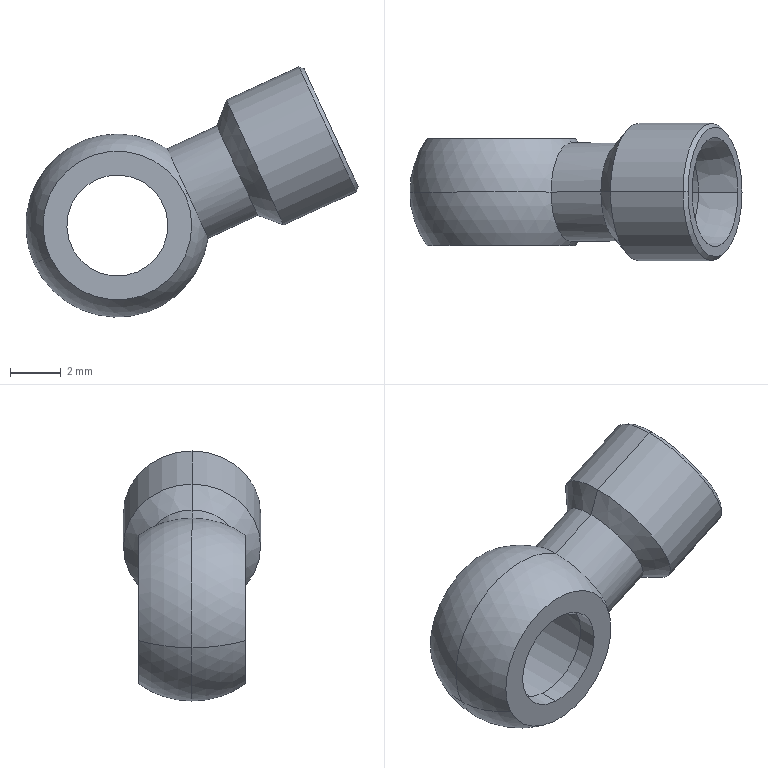Part | STEP file | 2026.6.15-Main Assembly图.sldasm-Part-257 | 1 solid | 31 faces | box 13.063 x 5.4 x 9.839 mm | volume 145.21 mm3 | cylinder 14 | cone 8 | plane 5 | sphere 4 | commonest cylinder face diameters 3.975 x4 2.1 x2 3.66 x2 3.87 x2 4.875 x2 5.4 x2
STEP:
#1=CARTESIAN_POINT('',(-1613.628,1444.049,3409.35));
#2=VERTEX_POINT('',#1);
#3=CARTESIAN_POINT('',(-1612.823,1442.114,3407.591));
#4=VERTEX_POINT('',#3);
#5=CARTESIAN_POINT('',(-1613.628,1442.114,3409.35));
#6=DIRECTION('',(-0.9092,0.,-0.4163));
#7=DIRECTION('',(0.4163,0.,-0.9092));
#8=AXIS2_PLACEMENT_3D('',#5,#6,#7);
#9=CIRCLE('',#8,1.935);
#10=EDGE_CURVE('',#2,#4,#9,.T.);
#11=ORIENTED_EDGE('',*,*,#10,.T.);
#12=CARTESIAN_POINT('',(-1619.662,1442.114,3406.588));
#13=VERTEX_POINT('',#12);
#14=CARTESIAN_POINT('',(-1616.388,1442.114,3408.086));
#15=DIRECTION('',(0.,1.,0.));
#16=DIRECTION('',(1.,0.,0.));
#17=AXIS2_PLACEMENT_3D('',#14,#15,#16);
#18=CIRCLE('',#17,3.6);
#19=EDGE_CURVE('',#4,#13,#18,.T.);
#20=ORIENTED_EDGE('',*,*,#19,.T.);
#21=CARTESIAN_POINT('',(-1619.047,1444.214,3406.869));
#22=VERTEX_POINT('',#21);
#23=CARTESIAN_POINT('',(-1616.388,1442.114,3408.086));
#24=DIRECTION('',(0.4163,0.,-0.9092));
#25=DIRECTION('',(0.9092,0.,0.4163));
#26=AXIS2_PLACEMENT_3D('',#23,#24,#25);
#27=CIRCLE('',#26,3.6);
#28=EDGE_CURVE('',#13,#22,#27,.T.);
#29=ORIENTED_EDGE('',*,*,#28,.T.);
#30=CARTESIAN_POINT('',(-1613.73,1444.214,3409.304));
#31=VERTEX_POINT('',#30);
#32=CARTESIAN_POINT('',(-1616.388,1444.214,3408.086));
#33=DIRECTION('',(0.,-1.,0.));
#34=DIRECTION('',(0.0785,0.,0.9969));
#35=AXIS2_PLACEMENT_3D('',#32,#33,#34);
#36=CIRCLE('',#35,2.924);
#37=EDGE_CURVE('',#22,#31,#36,.T.);
#38=ORIENTED_EDGE('',*,*,#37,.T.);
#39=CARTESIAN_POINT('',(-1616.388,1442.114,3408.086));
#40=DIRECTION('',(-0.4163,0.,0.9092));
#41=DIRECTION('',(-0.9092,0.,-0.4163));
#42=AXIS2_PLACEMENT_3D('',#39,#40,#41);
#43=CIRCLE('',#42,3.6);
#44=EDGE_CURVE('',#2,#31,#43,.T.);
#45=ORIENTED_EDGE('',*,*,#44,.F.);
#46=EDGE_LOOP('',(#11,#20,#29,#38,#45));
#47=FACE_OUTER_BOUND('',#46,.T.);
#48=CARTESIAN_POINT('',(-1616.388,1442.114,3408.086));
#49=DIRECTION('',(0.,1.,0.));
#50=DIRECTION('',(0.9092,0.,0.4163));
#51=AXIS2_PLACEMENT_3D('',#48,#49,#50);
#52=SPHERICAL_SURFACE('',#51,3.6);
#53=ADVANCED_FACE('',(#47),#52,.T.);
#54=CARTESIAN_POINT('',(-1614.434,1442.114,3411.109));
#55=VERTEX_POINT('',#54);
#56=CARTESIAN_POINT('',(-1616.388,1442.114,3408.086));
#57=DIRECTION('',(0.,-1.,0.));
#58=DIRECTION('',(0.,0.,1.));
#59=AXIS2_PLACEMENT_3D('',#56,#57,#58);
#60=CIRCLE('',#59,3.6);
#61=EDGE_CURVE('',#55,#13,#60,.T.);
#62=ORIENTED_EDGE('',*,*,#61,.F.);
#63=CARTESIAN_POINT('',(-1613.628,1442.114,3409.35));
#64=DIRECTION('',(-0.9092,0.,-0.4163));
#65=DIRECTION('',(0.4163,0.,-0.9092));
#66=AXIS2_PLACEMENT_3D('',#63,#64,#65);
#67=CIRCLE('',#66,1.935);
#68=EDGE_CURVE('',#55,#2,#67,.T.);
#69=ORIENTED_EDGE('',*,*,#68,.T.);
#70=ORIENTED_EDGE('',*,*,#44,.T.);
#71=CARTESIAN_POINT('',(-1616.388,1444.214,3408.086));
#72=DIRECTION('',(0.,-1.,0.));
#73=DIRECTION('',(0.0785,0.,0.9969));
#74=AXIS2_PLACEMENT_3D('',#71,#72,#73);
#75=CIRCLE('',#74,2.924);
#76=EDGE_CURVE('',#31,#22,#75,.T.);
#77=ORIENTED_EDGE('',*,*,#76,.T.);
#78=ORIENTED_EDGE('',*,*,#28,.F.);
#79=EDGE_LOOP('',(#62,#69,#70,#77,#78));
#80=FACE_OUTER_BOUND('',#79,.T.);
#81=CARTESIAN_POINT('',(-1616.388,1442.114,3408.086));
#82=DIRECTION('',(0.,1.,0.));
#83=DIRECTION('',(0.9092,0.,0.4163));
#84=AXIS2_PLACEMENT_3D('',#81,#82,#83);
#85=SPHERICAL_SURFACE('',#84,3.6);
#86=ADVANCED_FACE('',(#80),#85,.T.);
#87=CARTESIAN_POINT('',(-1611.067,1442.114,3412.535));
#88=VERTEX_POINT('',#87);
#89=CARTESIAN_POINT('',(-1610.16,1442.114,3412.95));
#90=VERTEX_POINT('',#89);
#91=CARTESIAN_POINT('',(-1610.16,1442.114,3412.95));
#92=DIRECTION('',(0.9092,0.,0.4163));
#93=VECTOR('',#92,1000.);
#94=LINE('',#91,#93);
#95=EDGE_CURVE('',#88,#90,#94,.T.);
#96=ORIENTED_EDGE('',*,*,#95,.F.);
#97=CARTESIAN_POINT('',(-1609.544,1442.114,3409.207));
#98=VERTEX_POINT('',#97);
#99=CARTESIAN_POINT('',(-1610.305,1442.114,3410.871));
#100=DIRECTION('',(-0.9092,0.,-0.4163));
#101=DIRECTION('',(0.4163,0.,-0.9092));
#102=AXIS2_PLACEMENT_3D('',#99,#100,#101);
#103=CIRCLE('',#102,1.83);
#104=EDGE_CURVE('',#88,#98,#103,.T.);
#105=ORIENTED_EDGE('',*,*,#104,.T.);
#106=CARTESIAN_POINT('',(-1608.637,1442.114,3409.623));
#107=VERTEX_POINT('',#106);
#108=CARTESIAN_POINT('',(-1608.637,1442.114,3409.623));
#109=DIRECTION('',(0.9092,0.,0.4163));
#110=VECTOR('',#109,1000.);
#111=LINE('',#108,#110);
#112=EDGE_CURVE('',#98,#107,#111,.T.);
#113=ORIENTED_EDGE('',*,*,#112,.T.);
#114=CARTESIAN_POINT('',(-1609.399,1442.114,3411.286));
#115=DIRECTION('',(0.9092,0.,0.4163));
#116=DIRECTION('',(0.4163,0.,-0.9092));
#117=AXIS2_PLACEMENT_3D('',#114,#115,#116);
#118=CIRCLE('',#117,1.83);
#119=EDGE_CURVE('',#107,#90,#118,.T.);
#120=ORIENTED_EDGE('',*,*,#119,.T.);
#121=EDGE_LOOP('',(#96,#105,#113,#120));
#122=FACE_OUTER_BOUND('',#121,.T.);
#123=CARTESIAN_POINT('',(-1609.399,1442.114,3411.286));
#124=DIRECTION('',(0.9092,0.,0.4163));
#125=DIRECTION('',(-0.4163,0.,0.9092));
#126=AXIS2_PLACEMENT_3D('',#123,#124,#125);
#127=CYLINDRICAL_SURFACE('',#126,1.83);
#128=ADVANCED_FACE('',(#122),#127,.F.);
#129=CARTESIAN_POINT('',(-1611.452,1442.114,3411.501));
#130=VERTEX_POINT('',#129);
#131=CARTESIAN_POINT('',(-1611.067,1442.114,3412.535));
#132=DIRECTION('',(0.3486,0.,0.9373));
#133=VECTOR('',#132,1000.);
#134=LINE('',#131,#133);
#135=EDGE_CURVE('',#130,#88,#134,.T.);
#136=ORIENTED_EDGE('',*,*,#135,.F.);
#137=CARTESIAN_POINT('',(-1610.578,1442.114,3409.592));
#138=VERTEX_POINT('',#137);
#139=CARTESIAN_POINT('',(-1611.015,1442.114,3410.547));
#140=DIRECTION('',(-0.9092,0.,-0.4163));
#141=DIRECTION('',(-0.4163,0.,0.9092));
#142=AXIS2_PLACEMENT_3D('',#139,#140,#141);
#143=CIRCLE('',#142,1.05);
#144=EDGE_CURVE('',#130,#138,#143,.T.);
#145=ORIENTED_EDGE('',*,*,#144,.T.);
#146=CARTESIAN_POINT('',(-1609.544,1442.114,3409.207));
#147=DIRECTION('',(0.9373,0.,-0.3486));
#148=VECTOR('',#147,1000.);
#149=LINE('',#146,#148);
#150=EDGE_CURVE('',#138,#98,#149,.T.);
#151=ORIENTED_EDGE('',*,*,#150,.T.);
#152=ORIENTED_EDGE('',*,*,#104,.F.);
#153=EDGE_LOOP('',(#136,#145,#151,#152));
#154=FACE_OUTER_BOUND('',#153,.T.);
#155=CARTESIAN_POINT('',(-1610.305,1442.114,3410.871));
#156=DIRECTION('',(0.9092,0.,0.4163));
#157=DIRECTION('',(-0.4163,0.,0.9092));
#158=AXIS2_PLACEMENT_3D('',#155,#156,#157);
#159=CONICAL_SURFACE('',#158,1.83,0.7854);
#160=ADVANCED_FACE('',(#154),#159,.F.);
#161=CARTESIAN_POINT('',(-1608.886,1442.114,3413.897));
#162=VERTEX_POINT('',#161);
#163=CARTESIAN_POINT('',(-1608.886,1442.114,3413.897));
#164=DIRECTION('',(0.8028,0.,0.5962));
#165=VECTOR('',#164,1000.);
#166=LINE('',#163,#165);
#167=EDGE_CURVE('',#90,#162,#166,.T.);
#168=ORIENTED_EDGE('',*,*,#167,.F.);
#169=ORIENTED_EDGE('',*,*,#119,.F.);
#170=CARTESIAN_POINT('',(-1607.088,1442.114,3409.969));
#171=VERTEX_POINT('',#170);
#172=CARTESIAN_POINT('',(-1607.088,1442.114,3409.969));
#173=DIRECTION('',(0.9759,0.,0.2181));
#174=VECTOR('',#173,1000.);
#175=LINE('',#172,#174);
#176=EDGE_CURVE('',#107,#171,#175,.T.);
#177=ORIENTED_EDGE('',*,*,#176,.T.);
#178=CARTESIAN_POINT('',(-1607.987,1442.114,3411.933));
#179=DIRECTION('',(-0.9092,0.,-0.4163));
#180=DIRECTION('',(0.4163,0.,-0.9092));
#181=AXIS2_PLACEMENT_3D('',#178,#179,#180);
#182=CIRCLE('',#181,2.16);
#183=EDGE_CURVE('',#162,#171,#182,.T.);
#184=ORIENTED_EDGE('',*,*,#183,.F.);
#185=EDGE_LOOP('',(#168,#169,#177,#184));
#186=FACE_OUTER_BOUND('',#185,.T.);
#187=CARTESIAN_POINT('',(-1607.987,1442.114,3411.933));
#188=DIRECTION('',(0.9092,0.,0.4163));
#189=DIRECTION('',(-0.4163,0.,0.9092));
#190=AXIS2_PLACEMENT_3D('',#187,#188,#189);
#191=CONICAL_SURFACE('',#190,2.16,0.2094);
#192=ADVANCED_FACE('',(#186),#191,.F.);
#193=CARTESIAN_POINT('',(-1613.951,1442.114,3408.047));
#194=VERTEX_POINT('',#193);
#195=CARTESIAN_POINT('',(-1621.807,1442.114,3404.451));
#196=DIRECTION('',(0.9092,0.,0.4163));
#197=VECTOR('',#196,1000.);
#198=LINE('',#195,#197);
#199=EDGE_CURVE('',#194,#138,#198,.T.);
#200=ORIENTED_EDGE('',*,*,#199,.T.);
#201=ORIENTED_EDGE('',*,*,#144,.F.);
#202=CARTESIAN_POINT('',(-1614.825,1442.114,3409.957));
#203=VERTEX_POINT('',#202);
#204=CARTESIAN_POINT('',(-1622.681,1442.114,3406.36));
#205=DIRECTION('',(0.9092,0.,0.4163));
#206=VECTOR('',#205,1000.);
#207=LINE('',#204,#206);
#208=EDGE_CURVE('',#203,#130,#207,.T.);
#209=ORIENTED_EDGE('',*,*,#208,.F.);
#210=CARTESIAN_POINT('',(-1614.825,1442.114,3409.957));
#211=CARTESIAN_POINT('',(-1614.825,1442.255,3409.957));
#212=CARTESIAN_POINT('',(-1614.801,1442.393,3409.937));
#213=CARTESIAN_POINT('',(-1614.715,1442.646,3409.86));
#214=CARTESIAN_POINT('',(-1614.654,1442.761,3409.802));
#215=CARTESIAN_POINT('',(-1614.519,1442.952,3409.654));
#216=CARTESIAN_POINT('',(-1614.444,1443.03,3409.561));
#217=CARTESIAN_POINT('',(-1614.3,1443.136,3409.35));
#218=CARTESIAN_POINT('',(-1614.231,1443.164,3409.229));
#219=CARTESIAN_POINT('',(-1614.115,1443.164,3408.976));
#220=CARTESIAN_POINT('',(-1614.068,1443.137,3408.845));
#221=CARTESIAN_POINT('',(-1614.001,1443.03,3408.594));
#222=CARTESIAN_POINT('',(-1613.98,1442.953,3408.478));
#223=CARTESIAN_POINT('',(-1613.956,1442.761,3408.278));
#224=CARTESIAN_POINT('',(-1613.952,1442.646,3408.194));
#225=CARTESIAN_POINT('',(-1613.95,1442.394,3408.079));
#226=CARTESIAN_POINT('',(-1613.951,1442.255,3408.047));
#227=CARTESIAN_POINT('',(-1613.951,1442.114,3408.047));
#228=B_SPLINE_CURVE_WITH_KNOTS('',3,(#210,#211,#212,#213,#214,#215,#216,#217,#218,#219,#220,#221,#222,#223,#224,#225,#226,#227),.UNSPECIFIED.,.F.,.F.,(4,2,2,2,2,2,2,2,4),(0.,0.0004153,0.0008305,0.001246,0.001661,0.002076,0.002492,0.002907,0.003322),.UNSPECIFIED.);
#229=EDGE_CURVE('',#203,#194,#228,.T.);
#230=ORIENTED_EDGE('',*,*,#229,.T.);
#231=EDGE_LOOP('',(#200,#201,#209,#230));
#232=FACE_OUTER_BOUND('',#231,.T.);
#233=CARTESIAN_POINT('',(-1622.244,1442.114,3405.405));
#234=DIRECTION('',(-0.9092,0.,-0.4163));
#235=DIRECTION('',(0.4163,0.,-0.9092));
#236=AXIS2_PLACEMENT_3D('',#233,#234,#235);
#237=CYLINDRICAL_SURFACE('',#236,1.05);
#238=ADVANCED_FACE('',(#232),#237,.F.);
#239=CARTESIAN_POINT('',(-1609.048,1442.114,3414.251));
#240=VERTEX_POINT('',#239);
#241=CARTESIAN_POINT('',(-1606.925,1442.114,3409.614));
#242=VERTEX_POINT('',#241);
#243=CARTESIAN_POINT('',(-1607.987,1442.114,3411.933));
#244=DIRECTION('',(-0.9092,0.,-0.4163));
#245=DIRECTION('',(-0.4163,0.,0.9092));
#246=AXIS2_PLACEMENT_3D('',#243,#244,#245);
#247=CIRCLE('',#246,2.55);
#248=EDGE_CURVE('',#240,#242,#247,.T.);
#249=ORIENTED_EDGE('',*,*,#248,.F.);
#250=CARTESIAN_POINT('',(-1607.987,1442.114,3411.933));
#251=DIRECTION('',(-0.9092,0.,-0.4163));
#252=DIRECTION('',(-0.4163,0.,0.9092));
#253=AXIS2_PLACEMENT_3D('',#250,#251,#252);
#254=CIRCLE('',#253,2.55);
#255=EDGE_CURVE('',#242,#240,#254,.T.);
#256=ORIENTED_EDGE('',*,*,#255,.F.);
#257=EDGE_LOOP('',(#249,#256));
#258=FACE_OUTER_BOUND('',#257,.T.);
#259=CARTESIAN_POINT('',(-1607.987,1442.114,3411.933));
#260=DIRECTION('',(-0.9092,0.,-0.4163));
#261=DIRECTION('',(0.4163,0.,-0.9092));
#262=AXIS2_PLACEMENT_3D('',#259,#260,#261);
#263=CIRCLE('',#262,2.16);
#264=EDGE_CURVE('',#171,#162,#263,.T.);
#265=ORIENTED_EDGE('',*,*,#264,.T.);
#266=ORIENTED_EDGE('',*,*,#183,.T.);
#267=EDGE_LOOP('',(#265,#266));
#268=FACE_BOUND('',#267,.T.);
#269=CARTESIAN_POINT('',(-1607.987,1444.814,3411.933));
#270=DIRECTION('',(0.9092,0.,0.4163));
#271=DIRECTION('',(-0.4163,0.,0.9092));
#272=AXIS2_PLACEMENT_3D('',#269,#270,#271);
#273=PLANE('',#272);
#274=ADVANCED_FACE('',(#258,#268),#273,.T.);
#275=CARTESIAN_POINT('',(-1616.197,1440.764,3410.516));
#276=VERTEX_POINT('',#275);
#277=CARTESIAN_POINT('',(-1616.197,1443.464,3410.516));
#278=VERTEX_POINT('',#277);
#279=CARTESIAN_POINT('',(-1616.197,1425.014,3410.516));
#280=DIRECTION('',(0.,1.,0.));
#281=VECTOR('',#280,1000.);
#282=LINE('',#279,#281);
#283=EDGE_CURVE('',#276,#278,#282,.T.);
#284=ORIENTED_EDGE('',*,*,#283,.F.);
#285=CARTESIAN_POINT('',(-1616.58,1440.764,3405.656));
#286=VERTEX_POINT('',#285);
#287=CARTESIAN_POINT('',(-1616.388,1440.764,3408.086));
#288=DIRECTION('',(0.,1.,0.));
#289=DIRECTION('',(-0.0785,0.,-0.9969));
#290=AXIS2_PLACEMENT_3D('',#287,#288,#289);
#291=CIRCLE('',#290,2.438);
#292=EDGE_CURVE('',#286,#276,#291,.T.);
#293=ORIENTED_EDGE('',*,*,#292,.F.);
#294=CARTESIAN_POINT('',(-1616.58,1443.464,3405.656));
#295=VERTEX_POINT('',#294);
#296=CARTESIAN_POINT('',(-1616.58,1425.014,3405.656));
#297=DIRECTION('',(0.,1.,0.));
#298=VECTOR('',#297,1000.);
#299=LINE('',#296,#298);
#300=EDGE_CURVE('',#286,#295,#299,.T.);
#301=ORIENTED_EDGE('',*,*,#300,.T.);
#302=CARTESIAN_POINT('',(-1616.388,1443.464,3408.086));
#303=DIRECTION('',(0.,-1.,0.));
#304=DIRECTION('',(-0.0785,0.,-0.9969));
#305=AXIS2_PLACEMENT_3D('',#302,#303,#304);
#306=CIRCLE('',#305,2.438);
#307=EDGE_CURVE('',#278,#295,#306,.T.);
#308=ORIENTED_EDGE('',*,*,#307,.F.);
#309=EDGE_LOOP('',(#284,#293,#301,#308));
#310=FACE_OUTER_BOUND('',#309,.T.);
#311=CARTESIAN_POINT('',(-1616.388,1425.014,3408.086));
#312=DIRECTION('',(0.,1.,0.));
#313=DIRECTION('',(0.0785,0.,0.9969));
#314=AXIS2_PLACEMENT_3D('',#311,#312,#313);
#315=CYLINDRICAL_SURFACE('',#314,2.438);
#316=ADVANCED_FACE('',(#310),#315,.F.);
#317=CARTESIAN_POINT('',(-1606.999,1442.114,3409.415));
#318=VERTEX_POINT('',#317);
#319=CARTESIAN_POINT('',(-1606.999,1442.114,3409.415));
#320=DIRECTION('',(0.3486,0.,0.9373));
#321=VECTOR('',#320,1000.);
#322=LINE('',#319,#321);
#323=EDGE_CURVE('',#318,#242,#322,.T.);
#324=ORIENTED_EDGE('',*,*,#323,.T.);
#325=ORIENTED_EDGE('',*,*,#255,.T.);
#326=CARTESIAN_POINT('',(-1609.247,1442.114,3414.325));
#327=VERTEX_POINT('',#326);
#328=CARTESIAN_POINT('',(-1609.247,1442.114,3414.325));
#329=DIRECTION('',(0.9373,0.,-0.3486));
#330=VECTOR('',#329,1000.);
#331=LINE('',#328,#330);
#332=EDGE_CURVE('',#327,#240,#331,.T.);
#333=ORIENTED_EDGE('',*,*,#332,.F.);
#334=CARTESIAN_POINT('',(-1608.123,1442.114,3411.87));
#335=DIRECTION('',(-0.9092,0.,-0.4163));
#336=DIRECTION('',(0.4163,0.,-0.9092));
#337=AXIS2_PLACEMENT_3D('',#334,#335,#336);
#338=CIRCLE('',#337,2.7);
#339=EDGE_CURVE('',#318,#327,#338,.T.);
#340=ORIENTED_EDGE('',*,*,#339,.F.);
#341=EDGE_LOOP('',(#324,#325,#333,#340));
#342=FACE_OUTER_BOUND('',#341,.T.);
#343=CARTESIAN_POINT('',(-1608.123,1442.114,3411.87));
#344=DIRECTION('',(-0.9092,0.,-0.4163));
#345=DIRECTION('',(0.4163,0.,-0.9092));
#346=AXIS2_PLACEMENT_3D('',#343,#344,#345);
#347=CONICAL_SURFACE('',#346,2.7,0.7854);
#348=ADVANCED_FACE('',(#342),#347,.T.);
#349=ORIENTED_EDGE('',*,*,#292,.T.);
#350=CARTESIAN_POINT('',(-1616.388,1440.764,3408.086));
#351=DIRECTION('',(0.,1.,0.));
#352=DIRECTION('',(-0.0785,0.,-0.9969));
#353=AXIS2_PLACEMENT_3D('',#350,#351,#352);
#354=CIRCLE('',#353,2.438);
#355=EDGE_CURVE('',#276,#286,#354,.T.);
#356=ORIENTED_EDGE('',*,*,#355,.T.);
#357=EDGE_LOOP('',(#349,#356));
#358=FACE_OUTER_BOUND('',#357,.T.);
#359=CARTESIAN_POINT('',(-1616.544,1440.764,3406.105));
#360=VERTEX_POINT('',#359);
#361=CARTESIAN_POINT('',(-1616.232,1440.764,3410.068));
#362=VERTEX_POINT('',#361);
#363=CARTESIAN_POINT('',(-1616.388,1440.764,3408.086));
#364=DIRECTION('',(0.,-1.,0.));
#365=DIRECTION('',(-0.0785,0.,-0.9969));
#366=AXIS2_PLACEMENT_3D('',#363,#364,#365);
#367=CIRCLE('',#366,1.987);
#368=EDGE_CURVE('',#360,#362,#367,.T.);
#369=ORIENTED_EDGE('',*,*,#368,.T.);
#370=CARTESIAN_POINT('',(-1616.388,1440.764,3408.086));
#371=DIRECTION('',(0.,-1.,0.));
#372=DIRECTION('',(-0.0785,0.,-0.9969));
#373=AXIS2_PLACEMENT_3D('',#370,#371,#372);
#374=CIRCLE('',#373,1.987);
#375=EDGE_CURVE('',#362,#360,#374,.T.);
#376=ORIENTED_EDGE('',*,*,#375,.T.);
#377=EDGE_LOOP('',(#369,#376));
#378=FACE_BOUND('',#377,.T.);
#379=CARTESIAN_POINT('',(-1617.403,1440.764,3410.303));
#380=DIRECTION('',(0.,1.,0.));
#381=DIRECTION('',(1.,0.,0.));
#382=AXIS2_PLACEMENT_3D('',#379,#380,#381);
#383=PLANE('',#382);
#384=ADVANCED_FACE('',(#358,#378),#383,.T.);
#385=CARTESIAN_POINT('',(-1616.388,1443.464,3408.086));
#386=DIRECTION('',(0.,-1.,0.));
#387=DIRECTION('',(-0.0785,0.,-0.9969));
#388=AXIS2_PLACEMENT_3D('',#385,#386,#387);
#389=CIRCLE('',#388,2.438);
#390=EDGE_CURVE('',#295,#278,#389,.T.);
#391=ORIENTED_EDGE('',*,*,#390,.T.);
#392=ORIENTED_EDGE('',*,*,#307,.T.);
#393=EDGE_LOOP('',(#391,#392));
#394=FACE_OUTER_BOUND('',#393,.T.);
#395=CARTESIAN_POINT('',(-1616.544,1443.464,3406.105));
#396=VERTEX_POINT('',#395);
#397=CARTESIAN_POINT('',(-1616.232,1443.464,3410.068));
#398=VERTEX_POINT('',#397);
#399=CARTESIAN_POINT('',(-1616.388,1443.464,3408.086));
#400=DIRECTION('',(0.,1.,0.));
#401=DIRECTION('',(-0.0785,0.,-0.9969));
#402=AXIS2_PLACEMENT_3D('',#399,#400,#401);
#403=CIRCLE('',#402,1.987);
#404=EDGE_CURVE('',#396,#398,#403,.T.);
#405=ORIENTED_EDGE('',*,*,#404,.T.);
#406=CARTESIAN_POINT('',(-1616.388,1443.464,3408.086));
#407=DIRECTION('',(0.,1.,0.));
#408=DIRECTION('',(-0.0785,0.,-0.9969));
#409=AXIS2_PLACEMENT_3D('',#406,#407,#408);
#410=CIRCLE('',#409,1.987);
#411=EDGE_CURVE('',#398,#396,#410,.T.);
#412=ORIENTED_EDGE('',*,*,#411,.T.);
#413=EDGE_LOOP('',(#405,#412));
#414=FACE_BOUND('',#413,.T.);
#415=CARTESIAN_POINT('',(-1617.216,1443.464,3409.893));
#416=DIRECTION('',(0.,-1.,0.));
#417=DIRECTION('',(0.,0.,-1.));
#418=AXIS2_PLACEMENT_3D('',#415,#416,#417);
#419=PLANE('',#418);
#420=ADVANCED_FACE('',(#394,#414),#419,.T.);
#421=CARTESIAN_POINT('',(-1612.098,1442.114,3413.02));
#422=VERTEX_POINT('',#421);
#423=CARTESIAN_POINT('',(-1633.878,1442.114,3403.048));
#424=DIRECTION('',(0.9092,0.,0.4163));
#425=VECTOR('',#424,1000.);
#426=LINE('',#423,#425);
#427=EDGE_CURVE('',#422,#327,#426,.T.);
#428=ORIENTED_EDGE('',*,*,#427,.F.);
#429=CARTESIAN_POINT('',(-1609.85,1442.114,3408.11));
#430=VERTEX_POINT('',#429);
#431=CARTESIAN_POINT('',(-1610.974,1442.114,3410.565));
#432=DIRECTION('',(-0.9092,0.,-0.4163));
#433=DIRECTION('',(0.4163,0.,-0.9092));
#434=AXIS2_PLACEMENT_3D('',#431,#432,#433);
#435=CIRCLE('',#434,2.7);
#436=EDGE_CURVE('',#430,#422,#435,.T.);
#437=ORIENTED_EDGE('',*,*,#436,.F.);
#438=CARTESIAN_POINT('',(-1631.631,1442.114,3398.138));
#439=DIRECTION('',(0.9092,0.,0.4163));
#440=VECTOR('',#439,1000.);
#441=LINE('',#438,#440);
#442=EDGE_CURVE('',#430,#318,#441,.T.);
#443=ORIENTED_EDGE('',*,*,#442,.T.);
#444=ORIENTED_EDGE('',*,*,#339,.T.);
#445=EDGE_LOOP('',(#428,#437,#443,#444));
#446=FACE_OUTER_BOUND('',#445,.T.);
#447=CARTESIAN_POINT('',(-1632.755,1442.114,3400.593));
#448=DIRECTION('',(0.9092,0.,0.4163));
#449=DIRECTION('',(-0.4163,0.,0.9092));
#450=AXIS2_PLACEMENT_3D('',#447,#448,#449);
#451=CYLINDRICAL_SURFACE('',#450,2.7);
#452=ADVANCED_FACE('',(#446),#451,.T.);
#453=CARTESIAN_POINT('',(-1616.232,1440.014,3410.068));
#454=VERTEX_POINT('',#453);
#455=CARTESIAN_POINT('',(-1616.232,1425.014,3410.068));
#456=DIRECTION('',(0.,1.,0.));
#457=VECTOR('',#456,1000.);
#458=LINE('',#455,#457);
#459=EDGE_CURVE('',#454,#362,#458,.T.);
#460=ORIENTED_EDGE('',*,*,#459,.F.);
#461=CARTESIAN_POINT('',(-1616.544,1440.014,3406.105));
#462=VERTEX_POINT('',#461);
#463=CARTESIAN_POINT('',(-1616.388,1440.014,3408.086));
#464=DIRECTION('',(0.,1.,0.));
#465=DIRECTION('',(-0.0785,0.,-0.9969));
#466=AXIS2_PLACEMENT_3D('',#463,#464,#465);
#467=CIRCLE('',#466,1.987);
#468=EDGE_CURVE('',#462,#454,#467,.T.);
#469=ORIENTED_EDGE('',*,*,#468,.F.);
#470=CARTESIAN_POINT('',(-1616.544,1425.014,3406.105));
#471=DIRECTION('',(0.,1.,0.));
#472=VECTOR('',#471,1000.);
#473=LINE('',#470,#472);
#474=EDGE_CURVE('',#462,#360,#473,.T.);
#475=ORIENTED_EDGE('',*,*,#474,.T.);
#476=ORIENTED_EDGE('',*,*,#375,.F.);
#477=EDGE_LOOP('',(#460,#469,#475,#476));
#478=FACE_OUTER_BOUND('',#477,.T.);
#479=CARTESIAN_POINT('',(-1616.388,1425.014,3408.086));
#480=DIRECTION('',(0.,1.,0.));
#481=DIRECTION('',(0.0785,0.,0.9969));
#482=AXIS2_PLACEMENT_3D('',#479,#480,#481);
#483=CYLINDRICAL_SURFACE('',#482,1.987);
#484=ADVANCED_FACE('',(#478),#483,.F.);
#485=CARTESIAN_POINT('',(-1616.232,1444.214,3410.068));
#486=VERTEX_POINT('',#485);
#487=CARTESIAN_POINT('',(-1616.232,1425.014,3410.068));
#488=DIRECTION('',(0.,1.,0.));
#489=VECTOR('',#488,1000.);
#490=LINE('',#487,#489);
#491=EDGE_CURVE('',#398,#486,#490,.T.);
#492=ORIENTED_EDGE('',*,*,#491,.F.);
#493=ORIENTED_EDGE('',*,*,#404,.F.);
#494=CARTESIAN_POINT('',(-1616.544,1444.214,3406.105));
#495=VERTEX_POINT('',#494);
#496=CARTESIAN_POINT('',(-1616.544,1425.014,3406.105));
#497=DIRECTION('',(0.,1.,0.));
#498=VECTOR('',#497,1000.);
#499=LINE('',#496,#498);
#500=EDGE_CURVE('',#396,#495,#499,.T.);
#501=ORIENTED_EDGE('',*,*,#500,.T.);
#502=CARTESIAN_POINT('',(-1616.388,1444.214,3408.086));
#503=DIRECTION('',(0.,-1.,0.));
#504=DIRECTION('',(-0.0785,0.,-0.9969));
#505=AXIS2_PLACEMENT_3D('',#502,#503,#504);
#506=CIRCLE('',#505,1.987);
#507=EDGE_CURVE('',#486,#495,#506,.T.);
#508=ORIENTED_EDGE('',*,*,#507,.F.);
#509=EDGE_LOOP('',(#492,#493,#501,#508));
#510=FACE_OUTER_BOUND('',#509,.T.);
#511=CARTESIAN_POINT('',(-1616.388,1425.014,3408.086));
#512=DIRECTION('',(0.,1.,0.));
#513=DIRECTION('',(0.0785,0.,0.9969));
#514=AXIS2_PLACEMENT_3D('',#511,#512,#513);
#515=CYLINDRICAL_SURFACE('',#514,1.987);
#516=ADVANCED_FACE('',(#510),#515,.F.);
#517=CARTESIAN_POINT('',(-1612.475,1442.114,3412.006));
#518=VERTEX_POINT('',#517);
#519=CARTESIAN_POINT('',(-1612.098,1442.114,3413.02));
#520=DIRECTION('',(0.3486,0.,0.9373));
#521=VECTOR('',#520,1000.);
#522=LINE('',#519,#521);
#523=EDGE_CURVE('',#518,#422,#522,.T.);
#524=ORIENTED_EDGE('',*,*,#523,.F.);
#525=CARTESIAN_POINT('',(-1610.864,1442.114,3408.487));
#526=VERTEX_POINT('',#525);
#527=CARTESIAN_POINT('',(-1611.669,1442.114,3410.247));
#528=DIRECTION('',(-0.9092,0.,-0.4163));
#529=DIRECTION('',(0.4163,0.,-0.9092));
#530=AXIS2_PLACEMENT_3D('',#527,#528,#529);
#531=CIRCLE('',#530,1.935);
#532=EDGE_CURVE('',#526,#518,#531,.T.);
#533=ORIENTED_EDGE('',*,*,#532,.F.);
#534=CARTESIAN_POINT('',(-1609.85,1442.114,3408.11));
#535=DIRECTION('',(0.9373,0.,-0.3486));
#536=VECTOR('',#535,1000.);
#537=LINE('',#534,#536);
#538=EDGE_CURVE('',#526,#430,#537,.T.);
#539=ORIENTED_EDGE('',*,*,#538,.T.);
#540=ORIENTED_EDGE('',*,*,#436,.T.);
#541=EDGE_LOOP('',(#524,#533,#539,#540));
#542=FACE_OUTER_BOUND('',#541,.T.);
#543=CARTESIAN_POINT('',(-1610.974,1442.114,3410.565));
#544=DIRECTION('',(0.9092,0.,0.4163));
#545=DIRECTION('',(-0.4163,0.,0.9092));
#546=AXIS2_PLACEMENT_3D('',#543,#544,#545);
#547=CONICAL_SURFACE('',#546,2.7,0.7854);
#548=ADVANCED_FACE('',(#542),#547,.T.);
#549=CARTESIAN_POINT('',(-1619.047,1440.014,3406.869));
#550=VERTEX_POINT('',#549);
#551=CARTESIAN_POINT('',(-1613.73,1440.014,3409.304));
#552=VERTEX_POINT('',#551);
#553=CARTESIAN_POINT('',(-1616.388,1440.014,3408.086));
#554=DIRECTION('',(0.,1.,0.));
#555=DIRECTION('',(0.0785,0.,0.9969));
#556=AXIS2_PLACEMENT_3D('',#553,#554,#555);
#557=CIRCLE('',#556,2.924);
#558=EDGE_CURVE('',#550,#552,#557,.T.);
#559=ORIENTED_EDGE('',*,*,#558,.F.);
#560=CARTESIAN_POINT('',(-1616.388,1440.014,3408.086));
#561=DIRECTION('',(0.,1.,0.));
#562=DIRECTION('',(0.0785,0.,0.9969));
#563=AXIS2_PLACEMENT_3D('',#560,#561,#562);
#564=CIRCLE('',#563,2.924);
#565=EDGE_CURVE('',#552,#550,#564,.T.);
#566=ORIENTED_EDGE('',*,*,#565,.F.);
#567=EDGE_LOOP('',(#559,#566));
#568=FACE_OUTER_BOUND('',#567,.T.);
#569=ORIENTED_EDGE('',*,*,#468,.T.);
#570=CARTESIAN_POINT('',(-1616.388,1440.014,3408.086));
#571=DIRECTION('',(0.,1.,0.));
#572=DIRECTION('',(-0.0785,0.,-0.9969));
#573=AXIS2_PLACEMENT_3D('',#570,#571,#572);
#574=CIRCLE('',#573,1.987);
#575=EDGE_CURVE('',#454,#462,#574,.T.);
#576=ORIENTED_EDGE('',*,*,#575,.T.);
#577=EDGE_LOOP('',(#569,#576));
#578=FACE_BOUND('',#577,.T.);
#579=CARTESIAN_POINT('',(-1616.38,1440.014,3427.607));
#580=DIRECTION('',(0.,-1.,0.));
#581=DIRECTION('',(0.,0.,-1.));
#582=AXIS2_PLACEMENT_3D('',#579,#580,#581);
#583=PLANE('',#582);
#584=ADVANCED_FACE('',(#568,#578),#583,.T.);
#585=ORIENTED_EDGE('',*,*,#37,.F.);
#586=ORIENTED_EDGE('',*,*,#76,.F.);
#587=EDGE_LOOP('',(#585,#586));
#588=FACE_OUTER_BOUND('',#587,.T.);
#589=CARTESIAN_POINT('',(-1616.388,1444.214,3408.086));
#590=DIRECTION('',(0.,-1.,0.));
#591=DIRECTION('',(-0.0785,0.,-0.9969));
#592=AXIS2_PLACEMENT_3D('',#589,#590,#591);
#593=CIRCLE('',#592,1.987);
#594=EDGE_CURVE('',#495,#486,#593,.T.);
#595=ORIENTED_EDGE('',*,*,#594,.T.);
#596=ORIENTED_EDGE('',*,*,#507,.T.);
#597=EDGE_LOOP('',(#595,#596));
#598=FACE_BOUND('',#597,.T.);
#599=CARTESIAN_POINT('',(-1630.41,1444.214,3421.775));
#600=DIRECTION('',(0.,1.,0.));
#601=DIRECTION('',(1.,0.,0.));
#602=AXIS2_PLACEMENT_3D('',#599,#600,#601);
#603=PLANE('',#602);
#604=ADVANCED_FACE('',(#588,#598),#603,.T.);
#605=CARTESIAN_POINT('',(-1633.56,1442.114,3402.353));
#606=DIRECTION('',(0.9092,0.,0.4163));
#607=VECTOR('',#606,1000.);
#608=LINE('',#605,#607);
#609=EDGE_CURVE('',#55,#518,#608,.T.);
#610=ORIENTED_EDGE('',*,*,#609,.F.);
#611=CARTESIAN_POINT('',(-1613.628,1440.179,3409.35));
#612=VERTEX_POINT('',#611);
#613=CARTESIAN_POINT('',(-1613.628,1442.114,3409.35));
#614=DIRECTION('',(-0.9092,0.,-0.4163));
#615=DIRECTION('',(0.4163,0.,-0.9092));
#616=AXIS2_PLACEMENT_3D('',#613,#614,#615);
#617=CIRCLE('',#616,1.935);
#618=EDGE_CURVE('',#612,#55,#617,.T.);
#619=ORIENTED_EDGE('',*,*,#618,.F.);
#620=CARTESIAN_POINT('',(-1613.628,1442.114,3409.35));
#621=DIRECTION('',(-0.9092,0.,-0.4163));
#622=DIRECTION('',(0.4163,0.,-0.9092));
#623=AXIS2_PLACEMENT_3D('',#620,#621,#622);
#624=CIRCLE('',#623,1.935);
#625=EDGE_CURVE('',#4,#612,#624,.T.);
#626=ORIENTED_EDGE('',*,*,#625,.F.);
#627=CARTESIAN_POINT('',(-1631.949,1442.114,3398.834));
#628=DIRECTION('',(0.9092,0.,0.4163));
#629=VECTOR('',#628,1000.);
#630=LINE('',#627,#629);
#631=EDGE_CURVE('',#4,#526,#630,.T.);
#632=ORIENTED_EDGE('',*,*,#631,.T.);
#633=ORIENTED_EDGE('',*,*,#532,.T.);
#634=EDGE_LOOP('',(#610,#619,#626,#632,#633));
#635=FACE_OUTER_BOUND('',#634,.T.);
#636=CARTESIAN_POINT('',(-1632.755,1442.114,3400.593));
#637=DIRECTION('',(0.9092,0.,0.4163));
#638=DIRECTION('',(-0.4163,0.,0.9092));
#639=AXIS2_PLACEMENT_3D('',#636,#637,#638);
#640=CYLINDRICAL_SURFACE('',#639,1.935);
#641=ADVANCED_FACE('',(#635),#640,.T.);
#642=ORIENTED_EDGE('',*,*,#618,.T.);
#643=ORIENTED_EDGE('',*,*,#61,.T.);
#644=CARTESIAN_POINT('',(-1616.388,1442.114,3408.086));
#645=DIRECTION('',(-0.4163,0.,0.9092));
#646=DIRECTION('',(0.9092,0.,0.4163));
#647=AXIS2_PLACEMENT_3D('',#644,#645,#646);
#648=CIRCLE('',#647,3.6);
#649=EDGE_CURVE('',#13,#550,#648,.T.);
#650=ORIENTED_EDGE('',*,*,#649,.T.);
#651=ORIENTED_EDGE('',*,*,#558,.T.);
#652=CARTESIAN_POINT('',(-1616.388,1442.114,3408.086));
#653=DIRECTION('',(0.4163,0.,-0.9092));
#654=DIRECTION('',(-0.9092,0.,-0.4163));
#655=AXIS2_PLACEMENT_3D('',#652,#653,#654);
#656=CIRCLE('',#655,3.6);
#657=EDGE_CURVE('',#612,#552,#656,.T.);
#658=ORIENTED_EDGE('',*,*,#657,.F.);
#659=EDGE_LOOP('',(#642,#643,#650,#651,#658));
#660=FACE_OUTER_BOUND('',#659,.T.);
#661=CARTESIAN_POINT('',(-1616.388,1442.114,3408.086));
#662=DIRECTION('',(0.,1.,0.));
#663=DIRECTION('',(0.9092,0.,0.4163));
#664=AXIS2_PLACEMENT_3D('',#661,#662,#663);
#665=SPHERICAL_SURFACE('',#664,3.6);
#666=ADVANCED_FACE('',(#660),#665,.T.);
#667=CARTESIAN_POINT('',(-1610.305,1442.114,3410.871));
#668=DIRECTION('',(-0.9092,0.,-0.4163));
#669=DIRECTION('',(0.4163,0.,-0.9092));
#670=AXIS2_PLACEMENT_3D('',#667,#668,#669);
#671=CIRCLE('',#670,1.83);
#672=EDGE_CURVE('',#98,#88,#671,.T.);
#673=ORIENTED_EDGE('',*,*,#672,.T.);
#674=ORIENTED_EDGE('',*,*,#95,.T.);
#675=CARTESIAN_POINT('',(-1609.399,1442.114,3411.286));
#676=DIRECTION('',(0.9092,0.,0.4163));
#677=DIRECTION('',(0.4163,0.,-0.9092));
#678=AXIS2_PLACEMENT_3D('',#675,#676,#677);
#679=CIRCLE('',#678,1.83);
#680=EDGE_CURVE('',#90,#107,#679,.T.);
#681=ORIENTED_EDGE('',*,*,#680,.T.);
#682=ORIENTED_EDGE('',*,*,#112,.F.);
#683=EDGE_LOOP('',(#673,#674,#681,#682));
#684=FACE_OUTER_BOUND('',#683,.T.);
#685=CARTESIAN_POINT('',(-1609.399,1442.114,3411.286));
#686=DIRECTION('',(0.9092,0.,0.4163));
#687=DIRECTION('',(-0.4163,0.,0.9092));
#688=AXIS2_PLACEMENT_3D('',#685,#686,#687);
#689=CYLINDRICAL_SURFACE('',#688,1.83);
#690=ADVANCED_FACE('',(#684),#689,.F.);
#691=CARTESIAN_POINT('',(-1611.015,1442.114,3410.547));
#692=DIRECTION('',(-0.9092,0.,-0.4163));
#693=DIRECTION('',(-0.4163,0.,0.9092));
#694=AXIS2_PLACEMENT_3D('',#691,#692,#693);
#695=CIRCLE('',#694,1.05);
#696=EDGE_CURVE('',#138,#130,#695,.T.);
#697=ORIENTED_EDGE('',*,*,#696,.T.);
#698=ORIENTED_EDGE('',*,*,#135,.T.);
#699=ORIENTED_EDGE('',*,*,#672,.F.);
#700=ORIENTED_EDGE('',*,*,#150,.F.);
#701=EDGE_LOOP('',(#697,#698,#699,#700));
#702=FACE_OUTER_BOUND('',#701,.T.);
#703=CARTESIAN_POINT('',(-1610.305,1442.114,3410.871));
#704=DIRECTION('',(0.9092,0.,0.4163));
#705=DIRECTION('',(-0.4163,0.,0.9092));
#706=AXIS2_PLACEMENT_3D('',#703,#704,#705);
#707=CONICAL_SURFACE('',#706,1.83,0.7854);
#708=ADVANCED_FACE('',(#702),#707,.F.);
#709=ORIENTED_EDGE('',*,*,#680,.F.);
#710=ORIENTED_EDGE('',*,*,#167,.T.);
#711=ORIENTED_EDGE('',*,*,#264,.F.);
#712=ORIENTED_EDGE('',*,*,#176,.F.);
#713=EDGE_LOOP('',(#709,#710,#711,#712));
#714=FACE_OUTER_BOUND('',#713,.T.);
#715=CARTESIAN_POINT('',(-1607.987,1442.114,3411.933));
#716=DIRECTION('',(0.9092,0.,0.4163));
#717=DIRECTION('',(-0.4163,0.,0.9092));
#718=AXIS2_PLACEMENT_3D('',#715,#716,#717);
#719=CONICAL_SURFACE('',#718,2.16,0.2094);
#720=ADVANCED_FACE('',(#714),#719,.F.);
#721=ORIENTED_EDGE('',*,*,#696,.F.);
#722=ORIENTED_EDGE('',*,*,#199,.F.);
#723=CARTESIAN_POINT('',(-1613.951,1442.114,3408.047));
#724=CARTESIAN_POINT('',(-1613.951,1441.974,3408.047));
#725=CARTESIAN_POINT('',(-1613.95,1441.836,3408.079));
#726=CARTESIAN_POINT('',(-1613.952,1441.583,3408.194));
#727=CARTESIAN_POINT('',(-1613.956,1441.468,3408.278));
#728=CARTESIAN_POINT('',(-1613.98,1441.277,3408.477));
#729=CARTESIAN_POINT('',(-1614.001,1441.199,3408.595));
#730=CARTESIAN_POINT('',(-1614.067,1441.093,3408.842));
#731=CARTESIAN_POINT('',(-1614.114,1441.064,3408.973));
#732=CARTESIAN_POINT('',(-1614.229,1441.064,3409.226));
#733=CARTESIAN_POINT('',(-1614.298,1441.092,3409.347));
#734=CARTESIAN_POINT('',(-1614.444,1441.199,3409.562));
#735=CARTESIAN_POINT('',(-1614.519,1441.276,3409.654));
#736=CARTESIAN_POINT('',(-1614.654,1441.468,3409.802));
#737=CARTESIAN_POINT('',(-1614.715,1441.583,3409.86));
#738=CARTESIAN_POINT('',(-1614.8,1441.835,3409.937));
#739=CARTESIAN_POINT('',(-1614.825,1441.974,3409.957));
#740=CARTESIAN_POINT('',(-1614.825,1442.114,3409.957));
#741=B_SPLINE_CURVE_WITH_KNOTS('',3,(#723,#724,#725,#726,#727,#728,#729,#730,#731,#732,#733,#734,#735,#736,#737,#738,#739,#740),.UNSPECIFIED.,.F.,.F.,(4,2,2,2,2,2,2,2,4),(0.,0.0004153,0.0008305,0.001246,0.001661,0.002076,0.002492,0.002907,0.003322),.UNSPECIFIED.);
#742=EDGE_CURVE('',#194,#203,#741,.T.);
#743=ORIENTED_EDGE('',*,*,#742,.T.);
#744=ORIENTED_EDGE('',*,*,#208,.T.);
#745=EDGE_LOOP('',(#721,#722,#743,#744));
#746=FACE_OUTER_BOUND('',#745,.T.);
#747=CARTESIAN_POINT('',(-1622.244,1442.114,3405.405));
#748=DIRECTION('',(-0.9092,0.,-0.4163));
#749=DIRECTION('',(0.4163,0.,-0.9092));
#750=AXIS2_PLACEMENT_3D('',#747,#748,#749);
#751=CYLINDRICAL_SURFACE('',#750,1.05);
#752=ADVANCED_FACE('',(#746),#751,.F.);
#753=ORIENTED_EDGE('',*,*,#355,.F.);
#754=ORIENTED_EDGE('',*,*,#283,.T.);
#755=ORIENTED_EDGE('',*,*,#390,.F.);
#756=ORIENTED_EDGE('',*,*,#300,.F.);
#757=EDGE_LOOP('',(#753,#754,#755,#756));
#758=FACE_OUTER_BOUND('',#757,.T.);
#759=ORIENTED_EDGE('',*,*,#229,.F.);
#760=ORIENTED_EDGE('',*,*,#742,.F.);
#761=EDGE_LOOP('',(#759,#760));
#762=FACE_BOUND('',#761,.T.);
#763=CARTESIAN_POINT('',(-1616.388,1425.014,3408.086));
#764=DIRECTION('',(0.,1.,0.));
#765=DIRECTION('',(0.0785,0.,0.9969));
#766=AXIS2_PLACEMENT_3D('',#763,#764,#765);
#767=CYLINDRICAL_SURFACE('',#766,2.438);
#768=ADVANCED_FACE('',(#758,#762),#767,.F.);
#769=ORIENTED_EDGE('',*,*,#248,.T.);
#770=ORIENTED_EDGE('',*,*,#323,.F.);
#771=CARTESIAN_POINT('',(-1608.123,1442.114,3411.87));
#772=DIRECTION('',(-0.9092,0.,-0.4163));
#773=DIRECTION('',(0.4163,0.,-0.9092));
#774=AXIS2_PLACEMENT_3D('',#771,#772,#773);
#775=CIRCLE('',#774,2.7);
#776=EDGE_CURVE('',#327,#318,#775,.T.);
#777=ORIENTED_EDGE('',*,*,#776,.F.);
#778=ORIENTED_EDGE('',*,*,#332,.T.);
#779=EDGE_LOOP('',(#769,#770,#777,#778));
#780=FACE_OUTER_BOUND('',#779,.T.);
#781=CARTESIAN_POINT('',(-1608.123,1442.114,3411.87));
#782=DIRECTION('',(-0.9092,0.,-0.4163));
#783=DIRECTION('',(0.4163,0.,-0.9092));
#784=AXIS2_PLACEMENT_3D('',#781,#782,#783);
#785=CONICAL_SURFACE('',#784,2.7,0.7854);
#786=ADVANCED_FACE('',(#780),#785,.T.);
#787=CARTESIAN_POINT('',(-1610.974,1442.114,3410.565));
#788=DIRECTION('',(-0.9092,0.,-0.4163));
#789=DIRECTION('',(0.4163,0.,-0.9092));
#790=AXIS2_PLACEMENT_3D('',#787,#788,#789);
#791=CIRCLE('',#790,2.7);
#792=EDGE_CURVE('',#422,#430,#791,.T.);
#793=ORIENTED_EDGE('',*,*,#792,.F.);
#794=ORIENTED_EDGE('',*,*,#427,.T.);
#795=ORIENTED_EDGE('',*,*,#776,.T.);
#796=ORIENTED_EDGE('',*,*,#442,.F.);
#797=EDGE_LOOP('',(#793,#794,#795,#796));
#798=FACE_OUTER_BOUND('',#797,.T.);
#799=CARTESIAN_POINT('',(-1632.755,1442.114,3400.593));
#800=DIRECTION('',(0.9092,0.,0.4163));
#801=DIRECTION('',(-0.4163,0.,0.9092));
#802=AXIS2_PLACEMENT_3D('',#799,#800,#801);
#803=CYLINDRICAL_SURFACE('',#802,2.7);
#804=ADVANCED_FACE('',(#798),#803,.T.);
#805=ORIENTED_EDGE('',*,*,#575,.F.);
#806=ORIENTED_EDGE('',*,*,#459,.T.);
#807=ORIENTED_EDGE('',*,*,#368,.F.);
#808=ORIENTED_EDGE('',*,*,#474,.F.);
#809=EDGE_LOOP('',(#805,#806,#807,#808));
#810=FACE_OUTER_BOUND('',#809,.T.);
#811=CARTESIAN_POINT('',(-1616.388,1425.014,3408.086));
#812=DIRECTION('',(0.,1.,0.));
#813=DIRECTION('',(0.0785,0.,0.9969));
#814=AXIS2_PLACEMENT_3D('',#811,#812,#813);
#815=CYLINDRICAL_SURFACE('',#814,1.987);
#816=ADVANCED_FACE('',(#810),#815,.F.);
#817=ORIENTED_EDGE('',*,*,#411,.F.);
#818=ORIENTED_EDGE('',*,*,#491,.T.);
#819=ORIENTED_EDGE('',*,*,#594,.F.);
#820=ORIENTED_EDGE('',*,*,#500,.F.);
#821=EDGE_LOOP('',(#817,#818,#819,#820));
#822=FACE_OUTER_BOUND('',#821,.T.);
#823=CARTESIAN_POINT('',(-1616.388,1425.014,3408.086));
#824=DIRECTION('',(0.,1.,0.));
#825=DIRECTION('',(0.0785,0.,0.9969));
#826=AXIS2_PLACEMENT_3D('',#823,#824,#825);
#827=CYLINDRICAL_SURFACE('',#826,1.987);
#828=ADVANCED_FACE('',(#822),#827,.F.);
#829=CARTESIAN_POINT('',(-1611.669,1442.114,3410.247));
#830=DIRECTION('',(-0.9092,0.,-0.4163));
#831=DIRECTION('',(0.4163,0.,-0.9092));
#832=AXIS2_PLACEMENT_3D('',#829,#830,#831);
#833=CIRCLE('',#832,1.935);
#834=EDGE_CURVE('',#518,#526,#833,.T.);
#835=ORIENTED_EDGE('',*,*,#834,.F.);
#836=ORIENTED_EDGE('',*,*,#523,.T.);
#837=ORIENTED_EDGE('',*,*,#792,.T.);
#838=ORIENTED_EDGE('',*,*,#538,.F.);
#839=EDGE_LOOP('',(#835,#836,#837,#838));
#840=FACE_OUTER_BOUND('',#839,.T.);
#841=CARTESIAN_POINT('',(-1610.974,1442.114,3410.565));
#842=DIRECTION('',(0.9092,0.,0.4163));
#843=DIRECTION('',(-0.4163,0.,0.9092));
#844=AXIS2_PLACEMENT_3D('',#841,#842,#843);
#845=CONICAL_SURFACE('',#844,2.7,0.7854);
#846=ADVANCED_FACE('',(#840),#845,.T.);
#847=ORIENTED_EDGE('',*,*,#68,.F.);
#848=ORIENTED_EDGE('',*,*,#609,.T.);
#849=ORIENTED_EDGE('',*,*,#834,.T.);
#850=ORIENTED_EDGE('',*,*,#631,.F.);
#851=ORIENTED_EDGE('',*,*,#10,.F.);
#852=EDGE_LOOP('',(#847,#848,#849,#850,#851));
#853=FACE_OUTER_BOUND('',#852,.T.);
#854=CARTESIAN_POINT('',(-1632.755,1442.114,3400.593));
#855=DIRECTION('',(0.9092,0.,0.4163));
#856=DIRECTION('',(-0.4163,0.,0.9092));
#857=AXIS2_PLACEMENT_3D('',#854,#855,#856);
#858=CYLINDRICAL_SURFACE('',#857,1.935);
#859=ADVANCED_FACE('',(#853),#858,.T.);
#860=ORIENTED_EDGE('',*,*,#19,.F.);
#861=ORIENTED_EDGE('',*,*,#625,.T.);
#862=ORIENTED_EDGE('',*,*,#657,.T.);
#863=ORIENTED_EDGE('',*,*,#565,.T.);
#864=ORIENTED_EDGE('',*,*,#649,.F.);
#865=EDGE_LOOP('',(#860,#861,#862,#863,#864));
#866=FACE_OUTER_BOUND('',#865,.T.);
#867=CARTESIAN_POINT('',(-1616.388,1442.114,3408.086));
#868=DIRECTION('',(0.,1.,0.));
#869=DIRECTION('',(0.9092,0.,0.4163));
#870=AXIS2_PLACEMENT_3D('',#867,#868,#869);
#871=SPHERICAL_SURFACE('',#870,3.6);
#872=ADVANCED_FACE('',(#866),#871,.T.);
#873=CLOSED_SHELL('',(#53,#86,#128,#160,#192,#238,#274,#316,#348,#384,#420,#452,#484,#516,#548,#584,#604,#641,#666,#690,#708,#720,#752,#768,#786,#804,#816,#828,#846,#859,#872));
#874=MANIFOLD_SOLID_BREP('',#873);
#875=CARTESIAN_POINT('',(0.,0.,0.));
#876=DIRECTION('',(0.,0.,1.));
#877=DIRECTION('',(1.,0.,0.));
#878=AXIS2_PLACEMENT_3D('',#875,#876,#877);
#879=(LENGTH_UNIT()NAMED_UNIT(*)SI_UNIT(.MILLI.,.METRE.));
#880=UNCERTAINTY_MEASURE_WITH_UNIT(LENGTH_MEASURE(0.00001),#879,'','');
#881=(NAMED_UNIT(*)PLANE_ANGLE_UNIT()SI_UNIT($,.RADIAN.));
#882=(NAMED_UNIT(*)SI_UNIT($,.STERADIAN.)SOLID_ANGLE_UNIT());
#883=(GEOMETRIC_REPRESENTATION_CONTEXT(3)GLOBAL_UNCERTAINTY_ASSIGNED_CONTEXT((#880))GLOBAL_UNIT_ASSIGNED_CONTEXT((#879,#881,#882))REPRESENTATION_CONTEXT('',''));
#884=ADVANCED_BREP_SHAPE_REPRESENTATION('',(#874,#878),#883);